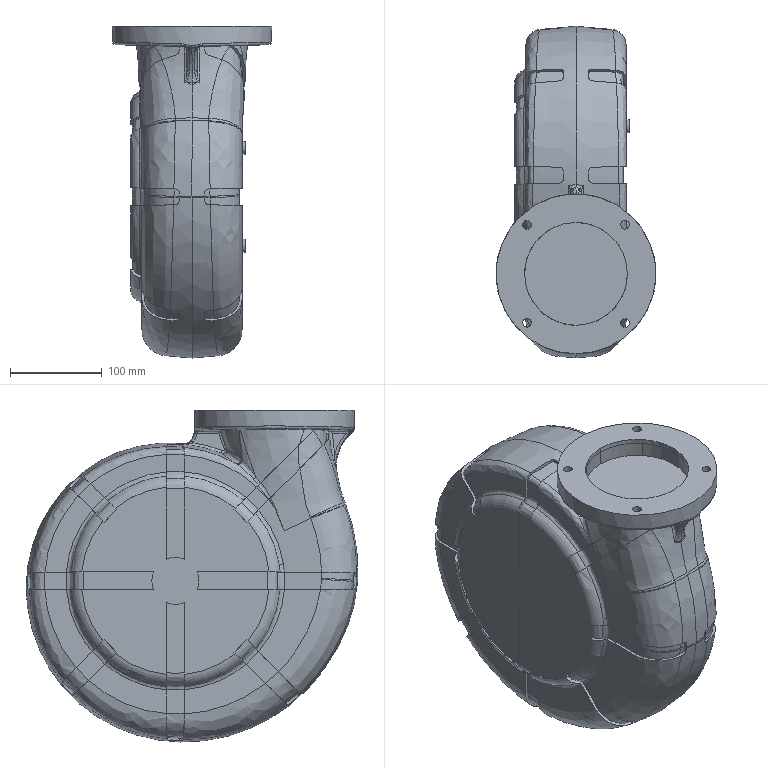Part | STEP file | a-hp_225_37-140_3_0_04 | 1 solid | 418 faces | box 174 x 361.133 x 361.501 mm | volume 10635738 mm3 | spline 185 | plane 139 | cylinder 70 | torus 20 | cone 4 | commonest cylinder face diameters 8 x30 201 x12 205 x8 6 x4 9.5 x4 14 x4